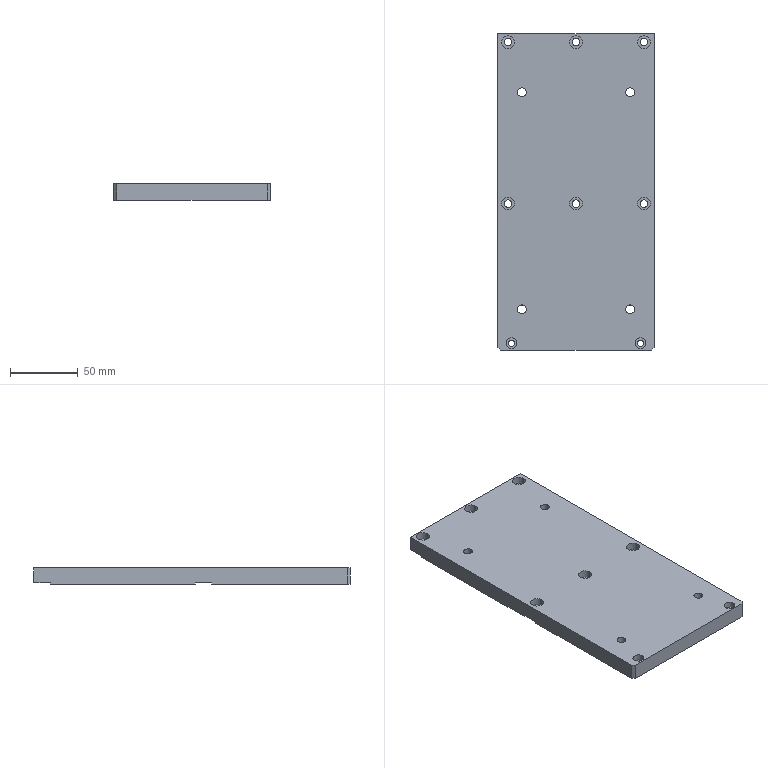Part | STEP file | PN_0001 Mount electronic clip base plate | 1 solid | 62 faces | box 115 x 233 x 12 mm | volume 313239 mm3 | cylinder 40 | plane 22 | commonest cylinder face diameters 5.5 x12 9.5 x12 6.5 x8 4.5 x4 8 x4